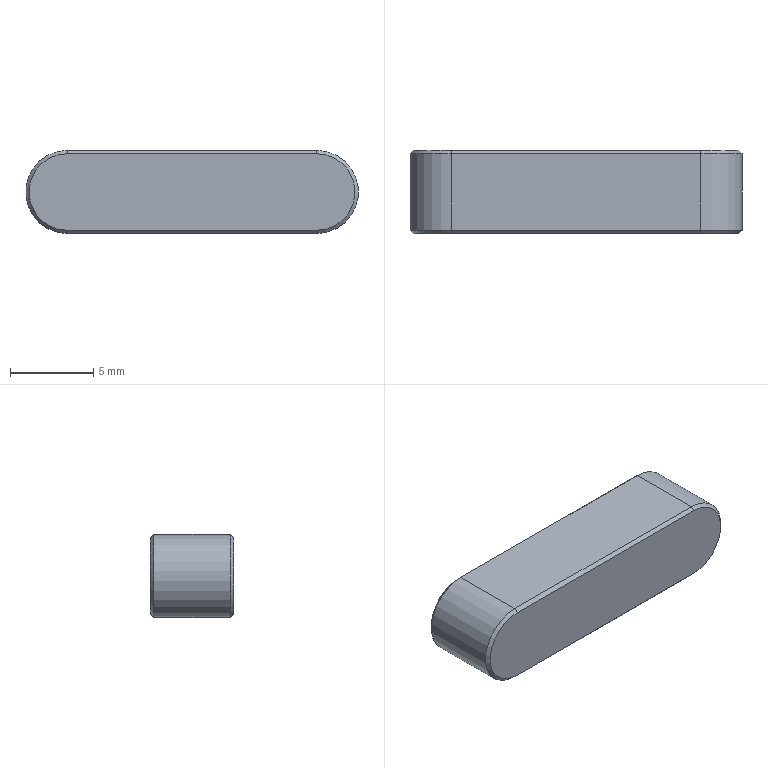Part | STEP file | 11-MISUMI-KES5-2011 | 1 solid | 14 faces | box 20 x 5 x 5 mm | volume 471.363 mm3 | plane 8 | cone 4 | cylinder 2 | commonest cylinder face diameters 5 x2
STEP:
#1=CARTESIAN_POINT('',(-7.5,4.8,-2.5));
#2=VERTEX_POINT('',#1);
#3=CARTESIAN_POINT('',(-7.5,0.2,-2.5));
#4=VERTEX_POINT('',#3);
#5=CARTESIAN_POINT('',(-7.5,5.,-2.5));
#6=DIRECTION('',(0.,-1.,0.));
#7=VECTOR('',#6,1000.);
#8=LINE('',#5,#7);
#9=EDGE_CURVE('',#2,#4,#8,.T.);
#10=ORIENTED_EDGE('',*,*,#9,.T.);
#11=CARTESIAN_POINT('',(-7.5,0.2,2.5));
#12=VERTEX_POINT('',#11);
#13=CARTESIAN_POINT('',(-7.5,0.2,0.));
#14=DIRECTION('',(0.,1.,0.));
#15=DIRECTION('',(0.,0.,1.));
#16=AXIS2_PLACEMENT_3D('',#13,#14,#15);
#17=CIRCLE('',#16,2.5);
#18=EDGE_CURVE('',#4,#12,#17,.T.);
#19=ORIENTED_EDGE('',*,*,#18,.T.);
#20=CARTESIAN_POINT('',(-7.5,4.8,2.5));
#21=VERTEX_POINT('',#20);
#22=CARTESIAN_POINT('',(-7.5,5.,2.5));
#23=DIRECTION('',(0.,-1.,0.));
#24=VECTOR('',#23,1000.);
#25=LINE('',#22,#24);
#26=EDGE_CURVE('',#21,#12,#25,.T.);
#27=ORIENTED_EDGE('',*,*,#26,.F.);
#28=CARTESIAN_POINT('',(-7.5,4.8,0.));
#29=DIRECTION('',(0.,-1.,0.));
#30=DIRECTION('',(0.,0.,1.));
#31=AXIS2_PLACEMENT_3D('',#28,#29,#30);
#32=CIRCLE('',#31,2.5);
#33=EDGE_CURVE('',#21,#2,#32,.T.);
#34=ORIENTED_EDGE('',*,*,#33,.T.);
#35=EDGE_LOOP('',(#10,#19,#27,#34));
#36=FACE_OUTER_BOUND('',#35,.T.);
#37=CARTESIAN_POINT('',(-7.5,5.,0.));
#38=DIRECTION('',(0.,-1.,0.));
#39=DIRECTION('',(0.,0.,-1.));
#40=AXIS2_PLACEMENT_3D('',#37,#38,#39);
#41=CYLINDRICAL_SURFACE('',#40,2.5);
#42=ADVANCED_FACE('',(#36),#41,.T.);
#43=ORIENTED_EDGE('',*,*,#26,.T.);
#44=CARTESIAN_POINT('',(7.5,0.2,2.5));
#45=VERTEX_POINT('',#44);
#46=CARTESIAN_POINT('',(-7.5,0.2,2.5));
#47=DIRECTION('',(1.,0.,0.));
#48=VECTOR('',#47,1000.);
#49=LINE('',#46,#48);
#50=EDGE_CURVE('',#12,#45,#49,.T.);
#51=ORIENTED_EDGE('',*,*,#50,.T.);
#52=CARTESIAN_POINT('',(7.5,4.8,2.5));
#53=VERTEX_POINT('',#52);
#54=CARTESIAN_POINT('',(7.5,5.,2.5));
#55=DIRECTION('',(0.,-1.,0.));
#56=VECTOR('',#55,1000.);
#57=LINE('',#54,#56);
#58=EDGE_CURVE('',#53,#45,#57,.T.);
#59=ORIENTED_EDGE('',*,*,#58,.F.);
#60=CARTESIAN_POINT('',(-7.5,4.8,2.5));
#61=DIRECTION('',(-1.,0.,0.));
#62=VECTOR('',#61,1000.);
#63=LINE('',#60,#62);
#64=EDGE_CURVE('',#53,#21,#63,.T.);
#65=ORIENTED_EDGE('',*,*,#64,.T.);
#66=EDGE_LOOP('',(#43,#51,#59,#65));
#67=FACE_OUTER_BOUND('',#66,.T.);
#68=CARTESIAN_POINT('',(-7.5,5.,2.5));
#69=DIRECTION('',(0.,0.,-1.));
#70=DIRECTION('',(-1.,0.,0.));
#71=AXIS2_PLACEMENT_3D('',#68,#69,#70);
#72=PLANE('',#71);
#73=ADVANCED_FACE('',(#67),#72,.F.);
#74=ORIENTED_EDGE('',*,*,#58,.T.);
#75=CARTESIAN_POINT('',(7.5,0.2,-2.5));
#76=VERTEX_POINT('',#75);
#77=CARTESIAN_POINT('',(7.5,0.2,0.));
#78=DIRECTION('',(0.,1.,0.));
#79=DIRECTION('',(0.,0.,1.));
#80=AXIS2_PLACEMENT_3D('',#77,#78,#79);
#81=CIRCLE('',#80,2.5);
#82=EDGE_CURVE('',#45,#76,#81,.T.);
#83=ORIENTED_EDGE('',*,*,#82,.T.);
#84=CARTESIAN_POINT('',(7.5,4.8,-2.5));
#85=VERTEX_POINT('',#84);
#86=CARTESIAN_POINT('',(7.5,5.,-2.5));
#87=DIRECTION('',(0.,-1.,0.));
#88=VECTOR('',#87,1000.);
#89=LINE('',#86,#88);
#90=EDGE_CURVE('',#85,#76,#89,.T.);
#91=ORIENTED_EDGE('',*,*,#90,.F.);
#92=CARTESIAN_POINT('',(7.5,4.8,0.));
#93=DIRECTION('',(0.,-1.,0.));
#94=DIRECTION('',(0.,0.,1.));
#95=AXIS2_PLACEMENT_3D('',#92,#93,#94);
#96=CIRCLE('',#95,2.5);
#97=EDGE_CURVE('',#85,#53,#96,.T.);
#98=ORIENTED_EDGE('',*,*,#97,.T.);
#99=EDGE_LOOP('',(#74,#83,#91,#98));
#100=FACE_OUTER_BOUND('',#99,.T.);
#101=CARTESIAN_POINT('',(7.5,5.,0.));
#102=DIRECTION('',(0.,-1.,0.));
#103=DIRECTION('',(0.,0.,-1.));
#104=AXIS2_PLACEMENT_3D('',#101,#102,#103);
#105=CYLINDRICAL_SURFACE('',#104,2.5);
#106=ADVANCED_FACE('',(#100),#105,.T.);
#107=ORIENTED_EDGE('',*,*,#90,.T.);
#108=CARTESIAN_POINT('',(-7.5,0.2,-2.5));
#109=DIRECTION('',(-1.,0.,0.));
#110=VECTOR('',#109,1000.);
#111=LINE('',#108,#110);
#112=EDGE_CURVE('',#76,#4,#111,.T.);
#113=ORIENTED_EDGE('',*,*,#112,.T.);
#114=ORIENTED_EDGE('',*,*,#9,.F.);
#115=CARTESIAN_POINT('',(7.5,4.8,-2.5));
#116=DIRECTION('',(1.,0.,0.));
#117=VECTOR('',#116,1000.);
#118=LINE('',#115,#117);
#119=EDGE_CURVE('',#2,#85,#118,.T.);
#120=ORIENTED_EDGE('',*,*,#119,.T.);
#121=EDGE_LOOP('',(#107,#113,#114,#120));
#122=FACE_OUTER_BOUND('',#121,.T.);
#123=CARTESIAN_POINT('',(-7.5,5.,-2.5));
#124=DIRECTION('',(0.,0.,1.));
#125=DIRECTION('',(1.,0.,0.));
#126=AXIS2_PLACEMENT_3D('',#123,#124,#125);
#127=PLANE('',#126);
#128=ADVANCED_FACE('',(#122),#127,.F.);
#129=CARTESIAN_POINT('',(7.5,5.,2.3));
#130=VERTEX_POINT('',#129);
#131=CARTESIAN_POINT('',(7.5,5.,-2.3));
#132=VERTEX_POINT('',#131);
#133=CARTESIAN_POINT('',(7.5,5.,0.));
#134=DIRECTION('',(0.,1.,0.));
#135=DIRECTION('',(0.,0.,1.));
#136=AXIS2_PLACEMENT_3D('',#133,#134,#135);
#137=CIRCLE('',#136,2.3);
#138=EDGE_CURVE('',#130,#132,#137,.T.);
#139=ORIENTED_EDGE('',*,*,#138,.T.);
#140=CARTESIAN_POINT('',(-7.5,5.,-2.3));
#141=VERTEX_POINT('',#140);
#142=CARTESIAN_POINT('',(-7.5,5.,-2.3));
#143=DIRECTION('',(-1.,0.,0.));
#144=VECTOR('',#143,1000.);
#145=LINE('',#142,#144);
#146=EDGE_CURVE('',#132,#141,#145,.T.);
#147=ORIENTED_EDGE('',*,*,#146,.T.);
#148=CARTESIAN_POINT('',(-7.5,5.,2.3));
#149=VERTEX_POINT('',#148);
#150=CARTESIAN_POINT('',(-7.5,5.,0.));
#151=DIRECTION('',(0.,1.,0.));
#152=DIRECTION('',(0.,0.,1.));
#153=AXIS2_PLACEMENT_3D('',#150,#151,#152);
#154=CIRCLE('',#153,2.3);
#155=EDGE_CURVE('',#141,#149,#154,.T.);
#156=ORIENTED_EDGE('',*,*,#155,.T.);
#157=CARTESIAN_POINT('',(7.5,5.,2.3));
#158=DIRECTION('',(1.,0.,0.));
#159=VECTOR('',#158,1000.);
#160=LINE('',#157,#159);
#161=EDGE_CURVE('',#149,#130,#160,.T.);
#162=ORIENTED_EDGE('',*,*,#161,.T.);
#163=EDGE_LOOP('',(#139,#147,#156,#162));
#164=FACE_OUTER_BOUND('',#163,.T.);
#165=CARTESIAN_POINT('',(-7.5,5.,0.));
#166=DIRECTION('',(0.,1.,0.));
#167=DIRECTION('',(0.,0.,1.));
#168=AXIS2_PLACEMENT_3D('',#165,#166,#167);
#169=PLANE('',#168);
#170=ADVANCED_FACE('',(#164),#169,.T.);
#171=CARTESIAN_POINT('',(7.5,0.,-2.3));
#172=VERTEX_POINT('',#171);
#173=CARTESIAN_POINT('',(7.5,0.,2.3));
#174=VERTEX_POINT('',#173);
#175=CARTESIAN_POINT('',(7.5,0.,0.));
#176=DIRECTION('',(0.,-1.,0.));
#177=DIRECTION('',(0.,0.,1.));
#178=AXIS2_PLACEMENT_3D('',#175,#176,#177);
#179=CIRCLE('',#178,2.3);
#180=EDGE_CURVE('',#172,#174,#179,.T.);
#181=ORIENTED_EDGE('',*,*,#180,.T.);
#182=CARTESIAN_POINT('',(-7.5,0.,2.3));
#183=VERTEX_POINT('',#182);
#184=CARTESIAN_POINT('',(-7.5,0.,2.3));
#185=DIRECTION('',(-1.,0.,0.));
#186=VECTOR('',#185,1000.);
#187=LINE('',#184,#186);
#188=EDGE_CURVE('',#174,#183,#187,.T.);
#189=ORIENTED_EDGE('',*,*,#188,.T.);
#190=CARTESIAN_POINT('',(-7.5,0.,-2.3));
#191=VERTEX_POINT('',#190);
#192=CARTESIAN_POINT('',(-7.5,0.,0.));
#193=DIRECTION('',(0.,-1.,0.));
#194=DIRECTION('',(0.,0.,1.));
#195=AXIS2_PLACEMENT_3D('',#192,#193,#194);
#196=CIRCLE('',#195,2.3);
#197=EDGE_CURVE('',#183,#191,#196,.T.);
#198=ORIENTED_EDGE('',*,*,#197,.T.);
#199=CARTESIAN_POINT('',(-7.5,0.,-2.3));
#200=DIRECTION('',(1.,0.,0.));
#201=VECTOR('',#200,1000.);
#202=LINE('',#199,#201);
#203=EDGE_CURVE('',#191,#172,#202,.T.);
#204=ORIENTED_EDGE('',*,*,#203,.T.);
#205=EDGE_LOOP('',(#181,#189,#198,#204));
#206=FACE_OUTER_BOUND('',#205,.T.);
#207=CARTESIAN_POINT('',(-7.5,0.,0.));
#208=DIRECTION('',(0.,1.,0.));
#209=DIRECTION('',(0.,0.,1.));
#210=AXIS2_PLACEMENT_3D('',#207,#208,#209);
#211=PLANE('',#210);
#212=ADVANCED_FACE('',(#206),#211,.F.);
#213=CARTESIAN_POINT('',(7.5,0.,-2.3));
#214=DIRECTION('',(0.,0.7071,-0.7071));
#215=VECTOR('',#214,1000.);
#216=LINE('',#213,#215);
#217=EDGE_CURVE('',#172,#76,#216,.T.);
#218=ORIENTED_EDGE('',*,*,#217,.F.);
#219=ORIENTED_EDGE('',*,*,#203,.F.);
#220=CARTESIAN_POINT('',(-7.5,0.2,-2.5));
#221=DIRECTION('',(0.,-0.7071,0.7071));
#222=VECTOR('',#221,1000.);
#223=LINE('',#220,#222);
#224=EDGE_CURVE('',#4,#191,#223,.T.);
#225=ORIENTED_EDGE('',*,*,#224,.F.);
#226=ORIENTED_EDGE('',*,*,#112,.F.);
#227=EDGE_LOOP('',(#218,#219,#225,#226));
#228=FACE_OUTER_BOUND('',#227,.T.);
#229=CARTESIAN_POINT('',(-7.5,0.2,-2.5));
#230=DIRECTION('',(0.,0.7071,0.7071));
#231=DIRECTION('',(0.,-0.7071,0.7071));
#232=AXIS2_PLACEMENT_3D('',#229,#230,#231);
#233=PLANE('',#232);
#234=ADVANCED_FACE('',(#228),#233,.F.);
#235=ORIENTED_EDGE('',*,*,#224,.T.);
#236=ORIENTED_EDGE('',*,*,#197,.F.);
#237=CARTESIAN_POINT('',(-7.5,0.2,2.5));
#238=DIRECTION('',(0.,-0.7071,-0.7071));
#239=VECTOR('',#238,1000.);
#240=LINE('',#237,#239);
#241=EDGE_CURVE('',#12,#183,#240,.T.);
#242=ORIENTED_EDGE('',*,*,#241,.F.);
#243=ORIENTED_EDGE('',*,*,#18,.F.);
#244=EDGE_LOOP('',(#235,#236,#242,#243));
#245=FACE_OUTER_BOUND('',#244,.T.);
#246=CARTESIAN_POINT('',(-7.5,0.2,0.));
#247=DIRECTION('',(0.,1.,0.));
#248=DIRECTION('',(0.,0.,1.));
#249=AXIS2_PLACEMENT_3D('',#246,#247,#248);
#250=CONICAL_SURFACE('',#249,2.5,0.7854);
#251=ADVANCED_FACE('',(#245),#250,.T.);
#252=ORIENTED_EDGE('',*,*,#217,.T.);
#253=ORIENTED_EDGE('',*,*,#82,.F.);
#254=CARTESIAN_POINT('',(7.5,0.,2.3));
#255=DIRECTION('',(0.,0.7071,0.7071));
#256=VECTOR('',#255,1000.);
#257=LINE('',#254,#256);
#258=EDGE_CURVE('',#174,#45,#257,.T.);
#259=ORIENTED_EDGE('',*,*,#258,.F.);
#260=ORIENTED_EDGE('',*,*,#180,.F.);
#261=EDGE_LOOP('',(#252,#253,#259,#260));
#262=FACE_OUTER_BOUND('',#261,.T.);
#263=CARTESIAN_POINT('',(7.5,0.2,0.));
#264=DIRECTION('',(0.,1.,0.));
#265=DIRECTION('',(0.,0.,1.));
#266=AXIS2_PLACEMENT_3D('',#263,#264,#265);
#267=CONICAL_SURFACE('',#266,2.5,0.7854);
#268=ADVANCED_FACE('',(#262),#267,.T.);
#269=ORIENTED_EDGE('',*,*,#241,.T.);
#270=ORIENTED_EDGE('',*,*,#188,.F.);
#271=ORIENTED_EDGE('',*,*,#258,.T.);
#272=ORIENTED_EDGE('',*,*,#50,.F.);
#273=EDGE_LOOP('',(#269,#270,#271,#272));
#274=FACE_OUTER_BOUND('',#273,.T.);
#275=CARTESIAN_POINT('',(-7.5,0.2,2.5));
#276=DIRECTION('',(0.,0.7071,-0.7071));
#277=DIRECTION('',(0.,0.7071,0.7071));
#278=AXIS2_PLACEMENT_3D('',#275,#276,#277);
#279=PLANE('',#278);
#280=ADVANCED_FACE('',(#274),#279,.F.);
#281=CARTESIAN_POINT('',(-7.5,4.8,2.5));
#282=DIRECTION('',(0.,0.7071,-0.7071));
#283=VECTOR('',#282,1000.);
#284=LINE('',#281,#283);
#285=EDGE_CURVE('',#21,#149,#284,.T.);
#286=ORIENTED_EDGE('',*,*,#285,.F.);
#287=ORIENTED_EDGE('',*,*,#64,.F.);
#288=CARTESIAN_POINT('',(7.5,5.,2.3));
#289=DIRECTION('',(0.,-0.7071,0.7071));
#290=VECTOR('',#289,1000.);
#291=LINE('',#288,#290);
#292=EDGE_CURVE('',#130,#53,#291,.T.);
#293=ORIENTED_EDGE('',*,*,#292,.F.);
#294=ORIENTED_EDGE('',*,*,#161,.F.);
#295=EDGE_LOOP('',(#286,#287,#293,#294));
#296=FACE_OUTER_BOUND('',#295,.T.);
#297=CARTESIAN_POINT('',(-7.5,5.,2.3));
#298=DIRECTION('',(0.,0.7071,0.7071));
#299=DIRECTION('',(0.,-0.7071,0.7071));
#300=AXIS2_PLACEMENT_3D('',#297,#298,#299);
#301=PLANE('',#300);
#302=ADVANCED_FACE('',(#296),#301,.T.);
#303=ORIENTED_EDGE('',*,*,#292,.T.);
#304=ORIENTED_EDGE('',*,*,#97,.F.);
#305=CARTESIAN_POINT('',(7.5,5.,-2.3));
#306=DIRECTION('',(0.,-0.7071,-0.7071));
#307=VECTOR('',#306,1000.);
#308=LINE('',#305,#307);
#309=EDGE_CURVE('',#132,#85,#308,.T.);
#310=ORIENTED_EDGE('',*,*,#309,.F.);
#311=ORIENTED_EDGE('',*,*,#138,.F.);
#312=EDGE_LOOP('',(#303,#304,#310,#311));
#313=FACE_OUTER_BOUND('',#312,.T.);
#314=CARTESIAN_POINT('',(7.5,5.,0.));
#315=DIRECTION('',(0.,-1.,0.));
#316=DIRECTION('',(0.,0.,-1.));
#317=AXIS2_PLACEMENT_3D('',#314,#315,#316);
#318=CONICAL_SURFACE('',#317,2.3,0.7854);
#319=ADVANCED_FACE('',(#313),#318,.T.);
#320=ORIENTED_EDGE('',*,*,#285,.T.);
#321=ORIENTED_EDGE('',*,*,#155,.F.);
#322=CARTESIAN_POINT('',(-7.5,4.8,-2.5));
#323=DIRECTION('',(0.,0.7071,0.7071));
#324=VECTOR('',#323,1000.);
#325=LINE('',#322,#324);
#326=EDGE_CURVE('',#2,#141,#325,.T.);
#327=ORIENTED_EDGE('',*,*,#326,.F.);
#328=ORIENTED_EDGE('',*,*,#33,.F.);
#329=EDGE_LOOP('',(#320,#321,#327,#328));
#330=FACE_OUTER_BOUND('',#329,.T.);
#331=CARTESIAN_POINT('',(-7.5,5.,0.));
#332=DIRECTION('',(0.,-1.,0.));
#333=DIRECTION('',(0.,0.,-1.));
#334=AXIS2_PLACEMENT_3D('',#331,#332,#333);
#335=CONICAL_SURFACE('',#334,2.3,0.7854);
#336=ADVANCED_FACE('',(#330),#335,.T.);
#337=ORIENTED_EDGE('',*,*,#309,.T.);
#338=ORIENTED_EDGE('',*,*,#119,.F.);
#339=ORIENTED_EDGE('',*,*,#326,.T.);
#340=ORIENTED_EDGE('',*,*,#146,.F.);
#341=EDGE_LOOP('',(#337,#338,#339,#340));
#342=FACE_OUTER_BOUND('',#341,.T.);
#343=CARTESIAN_POINT('',(-7.5,5.,-2.3));
#344=DIRECTION('',(0.,0.7071,-0.7071));
#345=DIRECTION('',(0.,0.7071,0.7071));
#346=AXIS2_PLACEMENT_3D('',#343,#344,#345);
#347=PLANE('',#346);
#348=ADVANCED_FACE('',(#342),#347,.T.);
#349=CLOSED_SHELL('',(#42,#73,#106,#128,#170,#212,#234,#251,#268,#280,#302,#319,#336,#348));
#350=MANIFOLD_SOLID_BREP('',#349);
#351=CARTESIAN_POINT('',(0.,0.,0.));
#352=DIRECTION('',(0.,0.,1.));
#353=DIRECTION('',(1.,0.,0.));
#354=AXIS2_PLACEMENT_3D('',#351,#352,#353);
#355=(LENGTH_UNIT()NAMED_UNIT(*)SI_UNIT(.MILLI.,.METRE.));
#356=UNCERTAINTY_MEASURE_WITH_UNIT(LENGTH_MEASURE(0.00001),#355,'','');
#357=(NAMED_UNIT(*)PLANE_ANGLE_UNIT()SI_UNIT($,.RADIAN.));
#358=(NAMED_UNIT(*)SI_UNIT($,.STERADIAN.)SOLID_ANGLE_UNIT());
#359=(GEOMETRIC_REPRESENTATION_CONTEXT(3)GLOBAL_UNCERTAINTY_ASSIGNED_CONTEXT((#356))GLOBAL_UNIT_ASSIGNED_CONTEXT((#355,#357,#358))REPRESENTATION_CONTEXT('',''));
#360=ADVANCED_BREP_SHAPE_REPRESENTATION('',(#350,#354),#359);